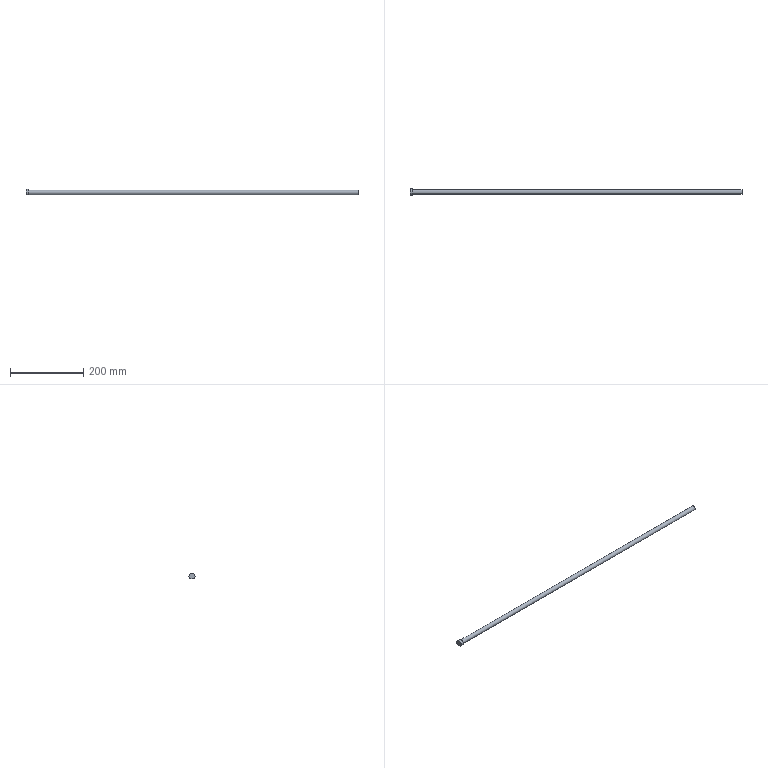Part | STEP file | solid 45 | 1 solid | 6 faces | box 905 x 17 x 15 mm | volume 103144 mm3 | plane 4 | cylinder 2 | commonest cylinder face diameters 12 x1 17 x1